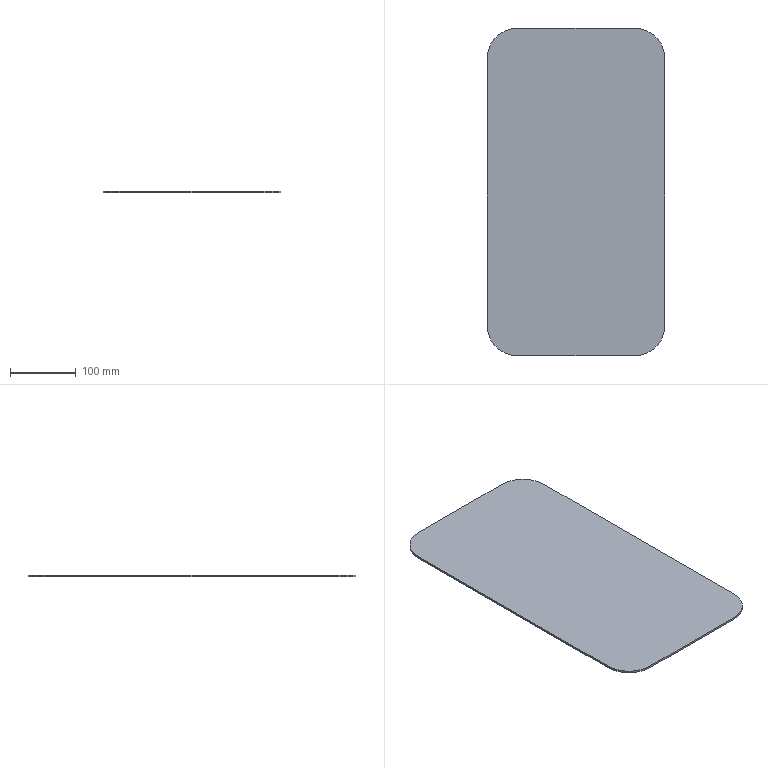Part | STEP file | Glass plate 1 | 1 solid | 10 faces | box 270 x 498 x 3 mm | volume 398165 mm3 | plane 6 | cylinder 4 | commonest cylinder face diameters 90 x4
STEP:
#1=CARTESIAN_POINT('',(0.,0.,0.));
#2=DIRECTION('',(0.,0.,1.));
#3=DIRECTION('',(1.,0.,0.));
#4=AXIS2_PLACEMENT_3D('',#1,#2,#3);
#5=CARTESIAN_POINT('',(-90.,249.,0.));
#6=VERTEX_POINT('',#5);
#7=CARTESIAN_POINT('',(-135.,204.,0.));
#8=VERTEX_POINT('',#7);
#9=CARTESIAN_POINT('',(-90.,204.,0.));
#10=DIRECTION('',(0.,0.,1.));
#11=DIRECTION('',(1.,0.,0.));
#12=AXIS2_PLACEMENT_3D('',#9,#10,#11);
#13=CIRCLE('',#12,45.);
#14=CARTESIAN_POINT('',(0.,0.,0.));
#15=DIRECTION('',(0.,0.,1.));
#16=DIRECTION('',(1.,0.,0.));
#17=AXIS2_PLACEMENT_3D('',#14,#15,#16);
#18=PLANE('',#17);
#19=CARTESIAN_POINT('',(-90.,204.));
#20=DIRECTION('',(1.,0.));
#21=AXIS2_PLACEMENT_2D('',#19,#20);
#22=CIRCLE('',#21,45.);
#23=(GEOMETRIC_REPRESENTATION_CONTEXT(2)PARAMETRIC_REPRESENTATION_CONTEXT()REPRESENTATION_CONTEXT('',''));
#24=DEFINITIONAL_REPRESENTATION('',(#22),#23);
#25=PCURVE('',#18,#24);
#26=CARTESIAN_POINT('',(-90.,204.,0.));
#27=DIRECTION('',(0.,0.,1.));
#28=DIRECTION('',(1.,0.,0.));
#29=AXIS2_PLACEMENT_3D('',#26,#27,#28);
#30=CYLINDRICAL_SURFACE('',#29,45.);
#31=CARTESIAN_POINT('',(0.,0.));
#32=DIRECTION('',(1.,0.));
#33=VECTOR('',#32,1.);
#34=LINE('',#31,#33);
#35=(GEOMETRIC_REPRESENTATION_CONTEXT(2)PARAMETRIC_REPRESENTATION_CONTEXT()REPRESENTATION_CONTEXT('',''));
#36=DEFINITIONAL_REPRESENTATION('',(#34),#35);
#37=PCURVE('',#30,#36);
#38=SURFACE_CURVE('',#13,(#25,#37),.PCURVE_S1.);
#39=EDGE_CURVE('',#6,#8,#38,.T.);
#40=ORIENTED_EDGE('',*,*,#39,.F.);
#41=CARTESIAN_POINT('',(90.,249.,0.));
#42=VERTEX_POINT('',#41);
#43=CARTESIAN_POINT('',(90.,249.,0.));
#44=DIRECTION('',(-1.,0.,0.));
#45=VECTOR('',#44,1.);
#46=LINE('',#43,#45);
#47=CARTESIAN_POINT('',(90.,249.));
#48=DIRECTION('',(-1.,0.));
#49=VECTOR('',#48,1.);
#50=LINE('',#47,#49);
#51=(GEOMETRIC_REPRESENTATION_CONTEXT(2)PARAMETRIC_REPRESENTATION_CONTEXT()REPRESENTATION_CONTEXT('',''));
#52=DEFINITIONAL_REPRESENTATION('',(#50),#51);
#53=PCURVE('',#18,#52);
#54=CARTESIAN_POINT('',(90.,249.,0.));
#55=DIRECTION('',(0.,1.,0.));
#56=DIRECTION('',(0.,0.,1.));
#57=AXIS2_PLACEMENT_3D('',#54,#55,#56);
#58=PLANE('',#57);
#59=CARTESIAN_POINT('',(0.,0.));
#60=DIRECTION('',(0.,-1.));
#61=VECTOR('',#60,1.);
#62=LINE('',#59,#61);
#63=(GEOMETRIC_REPRESENTATION_CONTEXT(2)PARAMETRIC_REPRESENTATION_CONTEXT()REPRESENTATION_CONTEXT('',''));
#64=DEFINITIONAL_REPRESENTATION('',(#62),#63);
#65=PCURVE('',#58,#64);
#66=SURFACE_CURVE('',#46,(#53,#65),.PCURVE_S1.);
#67=EDGE_CURVE('',#42,#6,#66,.T.);
#68=ORIENTED_EDGE('',*,*,#67,.F.);
#69=CARTESIAN_POINT('',(135.,204.,0.));
#70=VERTEX_POINT('',#69);
#71=CARTESIAN_POINT('',(90.,204.,0.));
#72=DIRECTION('',(0.,0.,1.));
#73=DIRECTION('',(1.,0.,0.));
#74=AXIS2_PLACEMENT_3D('',#71,#72,#73);
#75=CIRCLE('',#74,45.);
#76=CARTESIAN_POINT('',(90.,204.));
#77=DIRECTION('',(1.,0.));
#78=AXIS2_PLACEMENT_2D('',#76,#77);
#79=CIRCLE('',#78,45.);
#80=(GEOMETRIC_REPRESENTATION_CONTEXT(2)PARAMETRIC_REPRESENTATION_CONTEXT()REPRESENTATION_CONTEXT('',''));
#81=DEFINITIONAL_REPRESENTATION('',(#79),#80);
#82=PCURVE('',#18,#81);
#83=CARTESIAN_POINT('',(90.,204.,0.));
#84=DIRECTION('',(0.,0.,1.));
#85=DIRECTION('',(1.,0.,0.));
#86=AXIS2_PLACEMENT_3D('',#83,#84,#85);
#87=CYLINDRICAL_SURFACE('',#86,45.);
#88=CARTESIAN_POINT('',(0.,0.));
#89=DIRECTION('',(1.,0.));
#90=VECTOR('',#89,1.);
#91=LINE('',#88,#90);
#92=(GEOMETRIC_REPRESENTATION_CONTEXT(2)PARAMETRIC_REPRESENTATION_CONTEXT()REPRESENTATION_CONTEXT('',''));
#93=DEFINITIONAL_REPRESENTATION('',(#91),#92);
#94=PCURVE('',#87,#93);
#95=SURFACE_CURVE('',#75,(#82,#94),.PCURVE_S1.);
#96=EDGE_CURVE('',#70,#42,#95,.T.);
#97=ORIENTED_EDGE('',*,*,#96,.F.);
#98=CARTESIAN_POINT('',(135.,-204.,0.));
#99=VERTEX_POINT('',#98);
#100=CARTESIAN_POINT('',(135.,-204.,0.));
#101=DIRECTION('',(0.,1.,0.));
#102=VECTOR('',#101,1.);
#103=LINE('',#100,#102);
#104=CARTESIAN_POINT('',(135.,-204.));
#105=DIRECTION('',(0.,1.));
#106=VECTOR('',#105,1.);
#107=LINE('',#104,#106);
#108=(GEOMETRIC_REPRESENTATION_CONTEXT(2)PARAMETRIC_REPRESENTATION_CONTEXT()REPRESENTATION_CONTEXT('',''));
#109=DEFINITIONAL_REPRESENTATION('',(#107),#108);
#110=PCURVE('',#18,#109);
#111=CARTESIAN_POINT('',(135.,-204.,0.));
#112=DIRECTION('',(1.,0.,0.));
#113=DIRECTION('',(0.,0.,-1.));
#114=AXIS2_PLACEMENT_3D('',#111,#112,#113);
#115=PLANE('',#114);
#116=CARTESIAN_POINT('',(0.,0.));
#117=DIRECTION('',(0.,1.));
#118=VECTOR('',#117,1.);
#119=LINE('',#116,#118);
#120=(GEOMETRIC_REPRESENTATION_CONTEXT(2)PARAMETRIC_REPRESENTATION_CONTEXT()REPRESENTATION_CONTEXT('',''));
#121=DEFINITIONAL_REPRESENTATION('',(#119),#120);
#122=PCURVE('',#115,#121);
#123=SURFACE_CURVE('',#103,(#110,#122),.PCURVE_S1.);
#124=EDGE_CURVE('',#99,#70,#123,.T.);
#125=ORIENTED_EDGE('',*,*,#124,.F.);
#126=CARTESIAN_POINT('',(90.,-249.,0.));
#127=VERTEX_POINT('',#126);
#128=CARTESIAN_POINT('',(90.,-204.,0.));
#129=DIRECTION('',(0.,0.,1.));
#130=DIRECTION('',(1.,0.,0.));
#131=AXIS2_PLACEMENT_3D('',#128,#129,#130);
#132=CIRCLE('',#131,45.);
#133=CARTESIAN_POINT('',(90.,-204.));
#134=DIRECTION('',(1.,0.));
#135=AXIS2_PLACEMENT_2D('',#133,#134);
#136=CIRCLE('',#135,45.);
#137=(GEOMETRIC_REPRESENTATION_CONTEXT(2)PARAMETRIC_REPRESENTATION_CONTEXT()REPRESENTATION_CONTEXT('',''));
#138=DEFINITIONAL_REPRESENTATION('',(#136),#137);
#139=PCURVE('',#18,#138);
#140=CARTESIAN_POINT('',(90.,-204.,0.));
#141=DIRECTION('',(0.,0.,1.));
#142=DIRECTION('',(1.,0.,0.));
#143=AXIS2_PLACEMENT_3D('',#140,#141,#142);
#144=CYLINDRICAL_SURFACE('',#143,45.);
#145=CARTESIAN_POINT('',(0.,0.));
#146=DIRECTION('',(1.,0.));
#147=VECTOR('',#146,1.);
#148=LINE('',#145,#147);
#149=(GEOMETRIC_REPRESENTATION_CONTEXT(2)PARAMETRIC_REPRESENTATION_CONTEXT()REPRESENTATION_CONTEXT('',''));
#150=DEFINITIONAL_REPRESENTATION('',(#148),#149);
#151=PCURVE('',#144,#150);
#152=SURFACE_CURVE('',#132,(#139,#151),.PCURVE_S1.);
#153=EDGE_CURVE('',#127,#99,#152,.T.);
#154=ORIENTED_EDGE('',*,*,#153,.F.);
#155=CARTESIAN_POINT('',(-90.,-249.,0.));
#156=VERTEX_POINT('',#155);
#157=CARTESIAN_POINT('',(-90.,-249.,0.));
#158=DIRECTION('',(1.,0.,0.));
#159=VECTOR('',#158,1.);
#160=LINE('',#157,#159);
#161=CARTESIAN_POINT('',(-90.,-249.));
#162=DIRECTION('',(1.,0.));
#163=VECTOR('',#162,1.);
#164=LINE('',#161,#163);
#165=(GEOMETRIC_REPRESENTATION_CONTEXT(2)PARAMETRIC_REPRESENTATION_CONTEXT()REPRESENTATION_CONTEXT('',''));
#166=DEFINITIONAL_REPRESENTATION('',(#164),#165);
#167=PCURVE('',#18,#166);
#168=CARTESIAN_POINT('',(-90.,-249.,0.));
#169=DIRECTION('',(0.,-1.,0.));
#170=DIRECTION('',(0.,0.,-1.));
#171=AXIS2_PLACEMENT_3D('',#168,#169,#170);
#172=PLANE('',#171);
#173=CARTESIAN_POINT('',(0.,0.));
#174=DIRECTION('',(0.,1.));
#175=VECTOR('',#174,1.);
#176=LINE('',#173,#175);
#177=(GEOMETRIC_REPRESENTATION_CONTEXT(2)PARAMETRIC_REPRESENTATION_CONTEXT()REPRESENTATION_CONTEXT('',''));
#178=DEFINITIONAL_REPRESENTATION('',(#176),#177);
#179=PCURVE('',#172,#178);
#180=SURFACE_CURVE('',#160,(#167,#179),.PCURVE_S1.);
#181=EDGE_CURVE('',#156,#127,#180,.T.);
#182=ORIENTED_EDGE('',*,*,#181,.F.);
#183=CARTESIAN_POINT('',(-135.,-204.,0.));
#184=VERTEX_POINT('',#183);
#185=CARTESIAN_POINT('',(-90.,-204.,0.));
#186=DIRECTION('',(0.,0.,1.));
#187=DIRECTION('',(1.,0.,0.));
#188=AXIS2_PLACEMENT_3D('',#185,#186,#187);
#189=CIRCLE('',#188,45.);
#190=CARTESIAN_POINT('',(-90.,-204.));
#191=DIRECTION('',(1.,0.));
#192=AXIS2_PLACEMENT_2D('',#190,#191);
#193=CIRCLE('',#192,45.);
#194=(GEOMETRIC_REPRESENTATION_CONTEXT(2)PARAMETRIC_REPRESENTATION_CONTEXT()REPRESENTATION_CONTEXT('',''));
#195=DEFINITIONAL_REPRESENTATION('',(#193),#194);
#196=PCURVE('',#18,#195);
#197=CARTESIAN_POINT('',(-90.,-204.,0.));
#198=DIRECTION('',(0.,0.,1.));
#199=DIRECTION('',(1.,0.,0.));
#200=AXIS2_PLACEMENT_3D('',#197,#198,#199);
#201=CYLINDRICAL_SURFACE('',#200,45.);
#202=CARTESIAN_POINT('',(0.,0.));
#203=DIRECTION('',(1.,0.));
#204=VECTOR('',#203,1.);
#205=LINE('',#202,#204);
#206=(GEOMETRIC_REPRESENTATION_CONTEXT(2)PARAMETRIC_REPRESENTATION_CONTEXT()REPRESENTATION_CONTEXT('',''));
#207=DEFINITIONAL_REPRESENTATION('',(#205),#206);
#208=PCURVE('',#201,#207);
#209=SURFACE_CURVE('',#189,(#196,#208),.PCURVE_S1.);
#210=EDGE_CURVE('',#184,#156,#209,.T.);
#211=ORIENTED_EDGE('',*,*,#210,.F.);
#212=CARTESIAN_POINT('',(-135.,204.,0.));
#213=DIRECTION('',(0.,-1.,0.));
#214=VECTOR('',#213,1.);
#215=LINE('',#212,#214);
#216=CARTESIAN_POINT('',(-135.,204.));
#217=DIRECTION('',(0.,-1.));
#218=VECTOR('',#217,1.);
#219=LINE('',#216,#218);
#220=(GEOMETRIC_REPRESENTATION_CONTEXT(2)PARAMETRIC_REPRESENTATION_CONTEXT()REPRESENTATION_CONTEXT('',''));
#221=DEFINITIONAL_REPRESENTATION('',(#219),#220);
#222=PCURVE('',#18,#221);
#223=CARTESIAN_POINT('',(-135.,204.,0.));
#224=DIRECTION('',(-1.,0.,0.));
#225=DIRECTION('',(0.,0.,1.));
#226=AXIS2_PLACEMENT_3D('',#223,#224,#225);
#227=PLANE('',#226);
#228=CARTESIAN_POINT('',(0.,0.));
#229=DIRECTION('',(0.,-1.));
#230=VECTOR('',#229,1.);
#231=LINE('',#228,#230);
#232=(GEOMETRIC_REPRESENTATION_CONTEXT(2)PARAMETRIC_REPRESENTATION_CONTEXT()REPRESENTATION_CONTEXT('',''));
#233=DEFINITIONAL_REPRESENTATION('',(#231),#232);
#234=PCURVE('',#227,#233);
#235=SURFACE_CURVE('',#215,(#222,#234),.PCURVE_S1.);
#236=EDGE_CURVE('',#8,#184,#235,.T.);
#237=ORIENTED_EDGE('',*,*,#236,.F.);
#238=EDGE_LOOP('',(#40,#68,#97,#125,#154,#182,#211,#237));
#239=FACE_BOUND('',#238,.T.);
#240=ADVANCED_FACE('',(#239),#18,.F.);
#241=CARTESIAN_POINT('',(-90.,249.,3.));
#242=VERTEX_POINT('',#241);
#243=CARTESIAN_POINT('',(-135.,204.,3.));
#244=VERTEX_POINT('',#243);
#245=CARTESIAN_POINT('',(-90.,204.,3.));
#246=DIRECTION('',(0.,0.,1.));
#247=DIRECTION('',(1.,0.,0.));
#248=AXIS2_PLACEMENT_3D('',#245,#246,#247);
#249=CIRCLE('',#248,45.);
#250=CARTESIAN_POINT('',(0.,3.));
#251=DIRECTION('',(1.,0.));
#252=VECTOR('',#251,1.);
#253=LINE('',#250,#252);
#254=(GEOMETRIC_REPRESENTATION_CONTEXT(2)PARAMETRIC_REPRESENTATION_CONTEXT()REPRESENTATION_CONTEXT('',''));
#255=DEFINITIONAL_REPRESENTATION('',(#253),#254);
#256=PCURVE('',#30,#255);
#257=CARTESIAN_POINT('',(0.,0.,3.));
#258=DIRECTION('',(0.,0.,1.));
#259=DIRECTION('',(1.,0.,0.));
#260=AXIS2_PLACEMENT_3D('',#257,#258,#259);
#261=PLANE('',#260);
#262=CARTESIAN_POINT('',(-90.,204.));
#263=DIRECTION('',(1.,0.));
#264=AXIS2_PLACEMENT_2D('',#262,#263);
#265=CIRCLE('',#264,45.);
#266=(GEOMETRIC_REPRESENTATION_CONTEXT(2)PARAMETRIC_REPRESENTATION_CONTEXT()REPRESENTATION_CONTEXT('',''));
#267=DEFINITIONAL_REPRESENTATION('',(#265),#266);
#268=PCURVE('',#261,#267);
#269=SURFACE_CURVE('',#249,(#256,#268),.PCURVE_S1.);
#270=EDGE_CURVE('',#242,#244,#269,.T.);
#271=ORIENTED_EDGE('',*,*,#270,.F.);
#272=CARTESIAN_POINT('',(-90.,249.,0.));
#273=DIRECTION('',(0.,0.,1.));
#274=VECTOR('',#273,1.);
#275=LINE('',#272,#274);
#276=CARTESIAN_POINT('',(1.571,0.));
#277=DIRECTION('',(0.,1.));
#278=VECTOR('',#277,1.);
#279=LINE('',#276,#278);
#280=(GEOMETRIC_REPRESENTATION_CONTEXT(2)PARAMETRIC_REPRESENTATION_CONTEXT()REPRESENTATION_CONTEXT('',''));
#281=DEFINITIONAL_REPRESENTATION('',(#279),#280);
#282=PCURVE('',#30,#281);
#283=CARTESIAN_POINT('',(0.,-180.));
#284=DIRECTION('',(1.,0.));
#285=VECTOR('',#284,1.);
#286=LINE('',#283,#285);
#287=(GEOMETRIC_REPRESENTATION_CONTEXT(2)PARAMETRIC_REPRESENTATION_CONTEXT()REPRESENTATION_CONTEXT('',''));
#288=DEFINITIONAL_REPRESENTATION('',(#286),#287);
#289=PCURVE('',#58,#288);
#290=SURFACE_CURVE('',#275,(#282,#289),.PCURVE_S1.);
#291=EDGE_CURVE('',#6,#242,#290,.T.);
#292=ORIENTED_EDGE('',*,*,#291,.F.);
#293=ORIENTED_EDGE('',*,*,#39,.T.);
#294=CARTESIAN_POINT('',(-135.,204.,0.));
#295=DIRECTION('',(0.,0.,1.));
#296=VECTOR('',#295,1.);
#297=LINE('',#294,#296);
#298=CARTESIAN_POINT('',(3.142,0.));
#299=DIRECTION('',(0.,1.));
#300=VECTOR('',#299,1.);
#301=LINE('',#298,#300);
#302=(GEOMETRIC_REPRESENTATION_CONTEXT(2)PARAMETRIC_REPRESENTATION_CONTEXT()REPRESENTATION_CONTEXT('',''));
#303=DEFINITIONAL_REPRESENTATION('',(#301),#302);
#304=PCURVE('',#30,#303);
#305=CARTESIAN_POINT('',(0.,0.));
#306=DIRECTION('',(1.,0.));
#307=VECTOR('',#306,1.);
#308=LINE('',#305,#307);
#309=(GEOMETRIC_REPRESENTATION_CONTEXT(2)PARAMETRIC_REPRESENTATION_CONTEXT()REPRESENTATION_CONTEXT('',''));
#310=DEFINITIONAL_REPRESENTATION('',(#308),#309);
#311=PCURVE('',#227,#310);
#312=SURFACE_CURVE('',#297,(#304,#311),.PCURVE_S1.);
#313=EDGE_CURVE('',#8,#244,#312,.T.);
#314=ORIENTED_EDGE('',*,*,#313,.T.);
#315=EDGE_LOOP('',(#271,#292,#293,#314));
#316=FACE_BOUND('',#315,.T.);
#317=ADVANCED_FACE('',(#316),#30,.T.);
#318=CARTESIAN_POINT('',(90.,249.,3.));
#319=VERTEX_POINT('',#318);
#320=CARTESIAN_POINT('',(90.,249.,3.));
#321=DIRECTION('',(-1.,0.,0.));
#322=VECTOR('',#321,1.);
#323=LINE('',#320,#322);
#324=CARTESIAN_POINT('',(3.,0.));
#325=DIRECTION('',(0.,-1.));
#326=VECTOR('',#325,1.);
#327=LINE('',#324,#326);
#328=(GEOMETRIC_REPRESENTATION_CONTEXT(2)PARAMETRIC_REPRESENTATION_CONTEXT()REPRESENTATION_CONTEXT('',''));
#329=DEFINITIONAL_REPRESENTATION('',(#327),#328);
#330=PCURVE('',#58,#329);
#331=CARTESIAN_POINT('',(90.,249.));
#332=DIRECTION('',(-1.,0.));
#333=VECTOR('',#332,1.);
#334=LINE('',#331,#333);
#335=(GEOMETRIC_REPRESENTATION_CONTEXT(2)PARAMETRIC_REPRESENTATION_CONTEXT()REPRESENTATION_CONTEXT('',''));
#336=DEFINITIONAL_REPRESENTATION('',(#334),#335);
#337=PCURVE('',#261,#336);
#338=SURFACE_CURVE('',#323,(#330,#337),.PCURVE_S1.);
#339=EDGE_CURVE('',#319,#242,#338,.T.);
#340=ORIENTED_EDGE('',*,*,#339,.F.);
#341=CARTESIAN_POINT('',(90.,249.,0.));
#342=DIRECTION('',(0.,0.,1.));
#343=VECTOR('',#342,1.);
#344=LINE('',#341,#343);
#345=CARTESIAN_POINT('',(0.,0.));
#346=DIRECTION('',(1.,0.));
#347=VECTOR('',#346,1.);
#348=LINE('',#345,#347);
#349=(GEOMETRIC_REPRESENTATION_CONTEXT(2)PARAMETRIC_REPRESENTATION_CONTEXT()REPRESENTATION_CONTEXT('',''));
#350=DEFINITIONAL_REPRESENTATION('',(#348),#349);
#351=PCURVE('',#58,#350);
#352=CARTESIAN_POINT('',(1.571,0.));
#353=DIRECTION('',(0.,1.));
#354=VECTOR('',#353,1.);
#355=LINE('',#352,#354);
#356=(GEOMETRIC_REPRESENTATION_CONTEXT(2)PARAMETRIC_REPRESENTATION_CONTEXT()REPRESENTATION_CONTEXT('',''));
#357=DEFINITIONAL_REPRESENTATION('',(#355),#356);
#358=PCURVE('',#87,#357);
#359=SURFACE_CURVE('',#344,(#351,#358),.PCURVE_S1.);
#360=EDGE_CURVE('',#42,#319,#359,.T.);
#361=ORIENTED_EDGE('',*,*,#360,.F.);
#362=ORIENTED_EDGE('',*,*,#67,.T.);
#363=ORIENTED_EDGE('',*,*,#291,.T.);
#364=EDGE_LOOP('',(#340,#361,#362,#363));
#365=FACE_BOUND('',#364,.T.);
#366=ADVANCED_FACE('',(#365),#58,.T.);
#367=CARTESIAN_POINT('',(135.,204.,3.));
#368=VERTEX_POINT('',#367);
#369=CARTESIAN_POINT('',(90.,204.,3.));
#370=DIRECTION('',(0.,0.,1.));
#371=DIRECTION('',(1.,0.,0.));
#372=AXIS2_PLACEMENT_3D('',#369,#370,#371);
#373=CIRCLE('',#372,45.);
#374=CARTESIAN_POINT('',(0.,3.));
#375=DIRECTION('',(1.,0.));
#376=VECTOR('',#375,1.);
#377=LINE('',#374,#376);
#378=(GEOMETRIC_REPRESENTATION_CONTEXT(2)PARAMETRIC_REPRESENTATION_CONTEXT()REPRESENTATION_CONTEXT('',''));
#379=DEFINITIONAL_REPRESENTATION('',(#377),#378);
#380=PCURVE('',#87,#379);
#381=CARTESIAN_POINT('',(90.,204.));
#382=DIRECTION('',(1.,0.));
#383=AXIS2_PLACEMENT_2D('',#381,#382);
#384=CIRCLE('',#383,45.);
#385=(GEOMETRIC_REPRESENTATION_CONTEXT(2)PARAMETRIC_REPRESENTATION_CONTEXT()REPRESENTATION_CONTEXT('',''));
#386=DEFINITIONAL_REPRESENTATION('',(#384),#385);
#387=PCURVE('',#261,#386);
#388=SURFACE_CURVE('',#373,(#380,#387),.PCURVE_S1.);
#389=EDGE_CURVE('',#368,#319,#388,.T.);
#390=ORIENTED_EDGE('',*,*,#389,.F.);
#391=CARTESIAN_POINT('',(135.,204.,0.));
#392=DIRECTION('',(0.,0.,1.));
#393=VECTOR('',#392,1.);
#394=LINE('',#391,#393);
#395=CARTESIAN_POINT('',(0.,0.));
#396=DIRECTION('',(0.,1.));
#397=VECTOR('',#396,1.);
#398=LINE('',#395,#397);
#399=(GEOMETRIC_REPRESENTATION_CONTEXT(2)PARAMETRIC_REPRESENTATION_CONTEXT()REPRESENTATION_CONTEXT('',''));
#400=DEFINITIONAL_REPRESENTATION('',(#398),#399);
#401=PCURVE('',#87,#400);
#402=CARTESIAN_POINT('',(0.,408.));
#403=DIRECTION('',(-1.,0.));
#404=VECTOR('',#403,1.);
#405=LINE('',#402,#404);
#406=(GEOMETRIC_REPRESENTATION_CONTEXT(2)PARAMETRIC_REPRESENTATION_CONTEXT()REPRESENTATION_CONTEXT('',''));
#407=DEFINITIONAL_REPRESENTATION('',(#405),#406);
#408=PCURVE('',#115,#407);
#409=SURFACE_CURVE('',#394,(#401,#408),.PCURVE_S1.);
#410=EDGE_CURVE('',#70,#368,#409,.T.);
#411=ORIENTED_EDGE('',*,*,#410,.F.);
#412=ORIENTED_EDGE('',*,*,#96,.T.);
#413=ORIENTED_EDGE('',*,*,#360,.T.);
#414=EDGE_LOOP('',(#390,#411,#412,#413));
#415=FACE_BOUND('',#414,.T.);
#416=ADVANCED_FACE('',(#415),#87,.T.);
#417=CARTESIAN_POINT('',(135.,-204.,3.));
#418=VERTEX_POINT('',#417);
#419=CARTESIAN_POINT('',(135.,-204.,3.));
#420=DIRECTION('',(0.,1.,0.));
#421=VECTOR('',#420,1.);
#422=LINE('',#419,#421);
#423=CARTESIAN_POINT('',(-3.,0.));
#424=DIRECTION('',(0.,1.));
#425=VECTOR('',#424,1.);
#426=LINE('',#423,#425);
#427=(GEOMETRIC_REPRESENTATION_CONTEXT(2)PARAMETRIC_REPRESENTATION_CONTEXT()REPRESENTATION_CONTEXT('',''));
#428=DEFINITIONAL_REPRESENTATION('',(#426),#427);
#429=PCURVE('',#115,#428);
#430=CARTESIAN_POINT('',(135.,-204.));
#431=DIRECTION('',(0.,1.));
#432=VECTOR('',#431,1.);
#433=LINE('',#430,#432);
#434=(GEOMETRIC_REPRESENTATION_CONTEXT(2)PARAMETRIC_REPRESENTATION_CONTEXT()REPRESENTATION_CONTEXT('',''));
#435=DEFINITIONAL_REPRESENTATION('',(#433),#434);
#436=PCURVE('',#261,#435);
#437=SURFACE_CURVE('',#422,(#429,#436),.PCURVE_S1.);
#438=EDGE_CURVE('',#418,#368,#437,.T.);
#439=ORIENTED_EDGE('',*,*,#438,.F.);
#440=CARTESIAN_POINT('',(135.,-204.,0.));
#441=DIRECTION('',(0.,0.,1.));
#442=VECTOR('',#441,1.);
#443=LINE('',#440,#442);
#444=CARTESIAN_POINT('',(0.,0.));
#445=DIRECTION('',(-1.,0.));
#446=VECTOR('',#445,1.);
#447=LINE('',#444,#446);
#448=(GEOMETRIC_REPRESENTATION_CONTEXT(2)PARAMETRIC_REPRESENTATION_CONTEXT()REPRESENTATION_CONTEXT('',''));
#449=DEFINITIONAL_REPRESENTATION('',(#447),#448);
#450=PCURVE('',#115,#449);
#451=CARTESIAN_POINT('',(6.283,0.));
#452=DIRECTION('',(0.,1.));
#453=VECTOR('',#452,1.);
#454=LINE('',#451,#453);
#455=(GEOMETRIC_REPRESENTATION_CONTEXT(2)PARAMETRIC_REPRESENTATION_CONTEXT()REPRESENTATION_CONTEXT('',''));
#456=DEFINITIONAL_REPRESENTATION('',(#454),#455);
#457=PCURVE('',#144,#456);
#458=SURFACE_CURVE('',#443,(#450,#457),.PCURVE_S1.);
#459=EDGE_CURVE('',#99,#418,#458,.T.);
#460=ORIENTED_EDGE('',*,*,#459,.F.);
#461=ORIENTED_EDGE('',*,*,#124,.T.);
#462=ORIENTED_EDGE('',*,*,#410,.T.);
#463=EDGE_LOOP('',(#439,#460,#461,#462));
#464=FACE_BOUND('',#463,.T.);
#465=ADVANCED_FACE('',(#464),#115,.T.);
#466=CARTESIAN_POINT('',(90.,-249.,3.));
#467=VERTEX_POINT('',#466);
#468=CARTESIAN_POINT('',(90.,-204.,3.));
#469=DIRECTION('',(0.,0.,1.));
#470=DIRECTION('',(1.,0.,0.));
#471=AXIS2_PLACEMENT_3D('',#468,#469,#470);
#472=CIRCLE('',#471,45.);
#473=CARTESIAN_POINT('',(0.,3.));
#474=DIRECTION('',(1.,0.));
#475=VECTOR('',#474,1.);
#476=LINE('',#473,#475);
#477=(GEOMETRIC_REPRESENTATION_CONTEXT(2)PARAMETRIC_REPRESENTATION_CONTEXT()REPRESENTATION_CONTEXT('',''));
#478=DEFINITIONAL_REPRESENTATION('',(#476),#477);
#479=PCURVE('',#144,#478);
#480=CARTESIAN_POINT('',(90.,-204.));
#481=DIRECTION('',(1.,0.));
#482=AXIS2_PLACEMENT_2D('',#480,#481);
#483=CIRCLE('',#482,45.);
#484=(GEOMETRIC_REPRESENTATION_CONTEXT(2)PARAMETRIC_REPRESENTATION_CONTEXT()REPRESENTATION_CONTEXT('',''));
#485=DEFINITIONAL_REPRESENTATION('',(#483),#484);
#486=PCURVE('',#261,#485);
#487=SURFACE_CURVE('',#472,(#479,#486),.PCURVE_S1.);
#488=EDGE_CURVE('',#467,#418,#487,.T.);
#489=ORIENTED_EDGE('',*,*,#488,.F.);
#490=CARTESIAN_POINT('',(90.,-249.,0.));
#491=DIRECTION('',(0.,0.,1.));
#492=VECTOR('',#491,1.);
#493=LINE('',#490,#492);
#494=CARTESIAN_POINT('',(4.712,0.));
#495=DIRECTION('',(0.,1.));
#496=VECTOR('',#495,1.);
#497=LINE('',#494,#496);
#498=(GEOMETRIC_REPRESENTATION_CONTEXT(2)PARAMETRIC_REPRESENTATION_CONTEXT()REPRESENTATION_CONTEXT('',''));
#499=DEFINITIONAL_REPRESENTATION('',(#497),#498);
#500=PCURVE('',#144,#499);
#501=CARTESIAN_POINT('',(0.,180.));
#502=DIRECTION('',(-1.,0.));
#503=VECTOR('',#502,1.);
#504=LINE('',#501,#503);
#505=(GEOMETRIC_REPRESENTATION_CONTEXT(2)PARAMETRIC_REPRESENTATION_CONTEXT()REPRESENTATION_CONTEXT('',''));
#506=DEFINITIONAL_REPRESENTATION('',(#504),#505);
#507=PCURVE('',#172,#506);
#508=SURFACE_CURVE('',#493,(#500,#507),.PCURVE_S1.);
#509=EDGE_CURVE('',#127,#467,#508,.T.);
#510=ORIENTED_EDGE('',*,*,#509,.F.);
#511=ORIENTED_EDGE('',*,*,#153,.T.);
#512=ORIENTED_EDGE('',*,*,#459,.T.);
#513=EDGE_LOOP('',(#489,#510,#511,#512));
#514=FACE_BOUND('',#513,.T.);
#515=ADVANCED_FACE('',(#514),#144,.T.);
#516=CARTESIAN_POINT('',(-90.,-249.,3.));
#517=VERTEX_POINT('',#516);
#518=CARTESIAN_POINT('',(-90.,-249.,3.));
#519=DIRECTION('',(1.,0.,0.));
#520=VECTOR('',#519,1.);
#521=LINE('',#518,#520);
#522=CARTESIAN_POINT('',(-3.,0.));
#523=DIRECTION('',(0.,1.));
#524=VECTOR('',#523,1.);
#525=LINE('',#522,#524);
#526=(GEOMETRIC_REPRESENTATION_CONTEXT(2)PARAMETRIC_REPRESENTATION_CONTEXT()REPRESENTATION_CONTEXT('',''));
#527=DEFINITIONAL_REPRESENTATION('',(#525),#526);
#528=PCURVE('',#172,#527);
#529=CARTESIAN_POINT('',(-90.,-249.));
#530=DIRECTION('',(1.,0.));
#531=VECTOR('',#530,1.);
#532=LINE('',#529,#531);
#533=(GEOMETRIC_REPRESENTATION_CONTEXT(2)PARAMETRIC_REPRESENTATION_CONTEXT()REPRESENTATION_CONTEXT('',''));
#534=DEFINITIONAL_REPRESENTATION('',(#532),#533);
#535=PCURVE('',#261,#534);
#536=SURFACE_CURVE('',#521,(#528,#535),.PCURVE_S1.);
#537=EDGE_CURVE('',#517,#467,#536,.T.);
#538=ORIENTED_EDGE('',*,*,#537,.F.);
#539=CARTESIAN_POINT('',(-90.,-249.,0.));
#540=DIRECTION('',(0.,0.,1.));
#541=VECTOR('',#540,1.);
#542=LINE('',#539,#541);
#543=CARTESIAN_POINT('',(0.,0.));
#544=DIRECTION('',(-1.,0.));
#545=VECTOR('',#544,1.);
#546=LINE('',#543,#545);
#547=(GEOMETRIC_REPRESENTATION_CONTEXT(2)PARAMETRIC_REPRESENTATION_CONTEXT()REPRESENTATION_CONTEXT('',''));
#548=DEFINITIONAL_REPRESENTATION('',(#546),#547);
#549=PCURVE('',#172,#548);
#550=CARTESIAN_POINT('',(4.712,0.));
#551=DIRECTION('',(0.,1.));
#552=VECTOR('',#551,1.);
#553=LINE('',#550,#552);
#554=(GEOMETRIC_REPRESENTATION_CONTEXT(2)PARAMETRIC_REPRESENTATION_CONTEXT()REPRESENTATION_CONTEXT('',''));
#555=DEFINITIONAL_REPRESENTATION('',(#553),#554);
#556=PCURVE('',#201,#555);
#557=SURFACE_CURVE('',#542,(#549,#556),.PCURVE_S1.);
#558=EDGE_CURVE('',#156,#517,#557,.T.);
#559=ORIENTED_EDGE('',*,*,#558,.F.);
#560=ORIENTED_EDGE('',*,*,#181,.T.);
#561=ORIENTED_EDGE('',*,*,#509,.T.);
#562=EDGE_LOOP('',(#538,#559,#560,#561));
#563=FACE_BOUND('',#562,.T.);
#564=ADVANCED_FACE('',(#563),#172,.T.);
#565=CARTESIAN_POINT('',(-135.,-204.,3.));
#566=VERTEX_POINT('',#565);
#567=CARTESIAN_POINT('',(-90.,-204.,3.));
#568=DIRECTION('',(0.,0.,1.));
#569=DIRECTION('',(1.,0.,0.));
#570=AXIS2_PLACEMENT_3D('',#567,#568,#569);
#571=CIRCLE('',#570,45.);
#572=CARTESIAN_POINT('',(0.,3.));
#573=DIRECTION('',(1.,0.));
#574=VECTOR('',#573,1.);
#575=LINE('',#572,#574);
#576=(GEOMETRIC_REPRESENTATION_CONTEXT(2)PARAMETRIC_REPRESENTATION_CONTEXT()REPRESENTATION_CONTEXT('',''));
#577=DEFINITIONAL_REPRESENTATION('',(#575),#576);
#578=PCURVE('',#201,#577);
#579=CARTESIAN_POINT('',(-90.,-204.));
#580=DIRECTION('',(1.,0.));
#581=AXIS2_PLACEMENT_2D('',#579,#580);
#582=CIRCLE('',#581,45.);
#583=(GEOMETRIC_REPRESENTATION_CONTEXT(2)PARAMETRIC_REPRESENTATION_CONTEXT()REPRESENTATION_CONTEXT('',''));
#584=DEFINITIONAL_REPRESENTATION('',(#582),#583);
#585=PCURVE('',#261,#584);
#586=SURFACE_CURVE('',#571,(#578,#585),.PCURVE_S1.);
#587=EDGE_CURVE('',#566,#517,#586,.T.);
#588=ORIENTED_EDGE('',*,*,#587,.F.);
#589=CARTESIAN_POINT('',(-135.,-204.,0.));
#590=DIRECTION('',(0.,0.,1.));
#591=VECTOR('',#590,1.);
#592=LINE('',#589,#591);
#593=CARTESIAN_POINT('',(3.142,0.));
#594=DIRECTION('',(0.,1.));
#595=VECTOR('',#594,1.);
#596=LINE('',#593,#595);
#597=(GEOMETRIC_REPRESENTATION_CONTEXT(2)PARAMETRIC_REPRESENTATION_CONTEXT()REPRESENTATION_CONTEXT('',''));
#598=DEFINITIONAL_REPRESENTATION('',(#596),#597);
#599=PCURVE('',#201,#598);
#600=CARTESIAN_POINT('',(0.,-408.));
#601=DIRECTION('',(1.,0.));
#602=VECTOR('',#601,1.);
#603=LINE('',#600,#602);
#604=(GEOMETRIC_REPRESENTATION_CONTEXT(2)PARAMETRIC_REPRESENTATION_CONTEXT()REPRESENTATION_CONTEXT('',''));
#605=DEFINITIONAL_REPRESENTATION('',(#603),#604);
#606=PCURVE('',#227,#605);
#607=SURFACE_CURVE('',#592,(#599,#606),.PCURVE_S1.);
#608=EDGE_CURVE('',#184,#566,#607,.T.);
#609=ORIENTED_EDGE('',*,*,#608,.F.);
#610=ORIENTED_EDGE('',*,*,#210,.T.);
#611=ORIENTED_EDGE('',*,*,#558,.T.);
#612=EDGE_LOOP('',(#588,#609,#610,#611));
#613=FACE_BOUND('',#612,.T.);
#614=ADVANCED_FACE('',(#613),#201,.T.);
#615=CARTESIAN_POINT('',(-135.,204.,3.));
#616=DIRECTION('',(0.,-1.,0.));
#617=VECTOR('',#616,1.);
#618=LINE('',#615,#617);
#619=CARTESIAN_POINT('',(3.,0.));
#620=DIRECTION('',(0.,-1.));
#621=VECTOR('',#620,1.);
#622=LINE('',#619,#621);
#623=(GEOMETRIC_REPRESENTATION_CONTEXT(2)PARAMETRIC_REPRESENTATION_CONTEXT()REPRESENTATION_CONTEXT('',''));
#624=DEFINITIONAL_REPRESENTATION('',(#622),#623);
#625=PCURVE('',#227,#624);
#626=CARTESIAN_POINT('',(-135.,204.));
#627=DIRECTION('',(0.,-1.));
#628=VECTOR('',#627,1.);
#629=LINE('',#626,#628);
#630=(GEOMETRIC_REPRESENTATION_CONTEXT(2)PARAMETRIC_REPRESENTATION_CONTEXT()REPRESENTATION_CONTEXT('',''));
#631=DEFINITIONAL_REPRESENTATION('',(#629),#630);
#632=PCURVE('',#261,#631);
#633=SURFACE_CURVE('',#618,(#625,#632),.PCURVE_S1.);
#634=EDGE_CURVE('',#244,#566,#633,.T.);
#635=ORIENTED_EDGE('',*,*,#634,.F.);
#636=ORIENTED_EDGE('',*,*,#313,.F.);
#637=ORIENTED_EDGE('',*,*,#236,.T.);
#638=ORIENTED_EDGE('',*,*,#608,.T.);
#639=EDGE_LOOP('',(#635,#636,#637,#638));
#640=FACE_BOUND('',#639,.T.);
#641=ADVANCED_FACE('',(#640),#227,.T.);
#642=ORIENTED_EDGE('',*,*,#339,.T.);
#643=ORIENTED_EDGE('',*,*,#270,.T.);
#644=ORIENTED_EDGE('',*,*,#634,.T.);
#645=ORIENTED_EDGE('',*,*,#587,.T.);
#646=ORIENTED_EDGE('',*,*,#537,.T.);
#647=ORIENTED_EDGE('',*,*,#488,.T.);
#648=ORIENTED_EDGE('',*,*,#438,.T.);
#649=ORIENTED_EDGE('',*,*,#389,.T.);
#650=EDGE_LOOP('',(#642,#643,#644,#645,#646,#647,#648,#649));
#651=FACE_BOUND('',#650,.T.);
#652=ADVANCED_FACE('',(#651),#261,.T.);
#653=CLOSED_SHELL('',(#240,#317,#366,#416,#465,#515,#564,#614,#641,#652));
#654=MANIFOLD_SOLID_BREP('',#653);
#655=(LENGTH_UNIT()NAMED_UNIT(*)SI_UNIT(.MILLI.,.METRE.));
#656=UNCERTAINTY_MEASURE_WITH_UNIT(LENGTH_MEASURE(0.0000001),#655,'','');
#657=(NAMED_UNIT(*)PLANE_ANGLE_UNIT()SI_UNIT($,.RADIAN.));
#658=(NAMED_UNIT(*)SI_UNIT($,.STERADIAN.)SOLID_ANGLE_UNIT());
#659=(GEOMETRIC_REPRESENTATION_CONTEXT(3)GLOBAL_UNCERTAINTY_ASSIGNED_CONTEXT((#656))GLOBAL_UNIT_ASSIGNED_CONTEXT((#655,#657,#658))REPRESENTATION_CONTEXT('',''));
#660=ADVANCED_BREP_SHAPE_REPRESENTATION('',(#4,#654),#659);